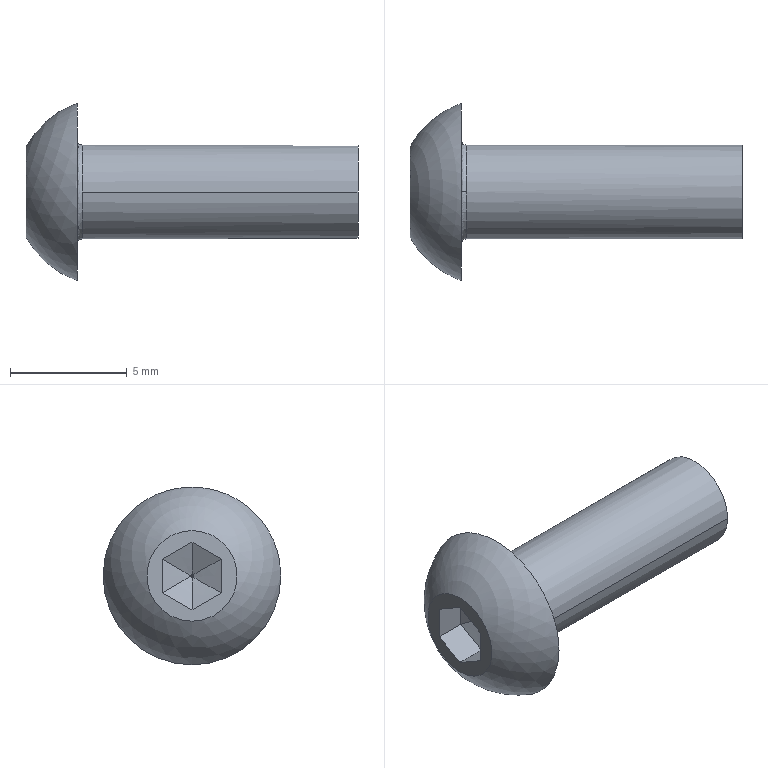Part | SolidWorks | features BaseBody 1 | 1 solid | 21 faces | box 14.2 x 7.6 x 7.6 mm | volume 211.112 mm3 | plane 10 | spline 8 | cylinder 2 | sphere 1 | commonest cylinder face diameters 4 x2